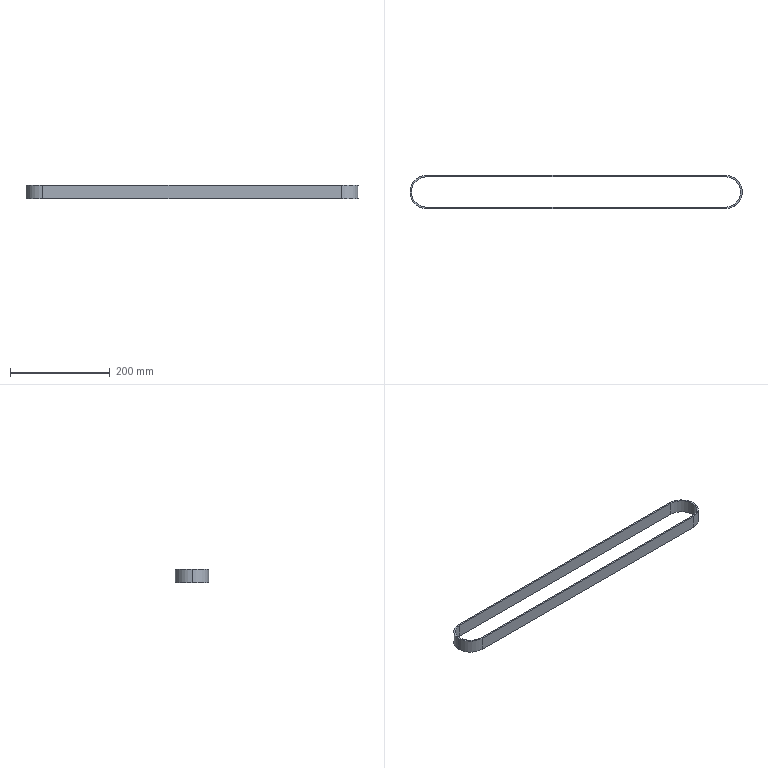Part | SolidWorks | features Extrusion 1 | 1 solid | 12 faces | box 667 x 67 x 27 mm | volume 113486 mm3 | cylinder 6 | plane 6 | commonest cylinder face diameters 61 x3 67 x3
STEP:
#1=CARTESIAN_POINT('',(0.,30.5,13.5));
#2=VERTEX_POINT('',#1);
#3=CARTESIAN_POINT('',(-30.5,0.,13.5));
#4=VERTEX_POINT('',#3);
#5=CARTESIAN_POINT('',(0.,0.,13.5));
#6=DIRECTION('',(0.,0.,1.));
#7=DIRECTION('',(1.,0.,0.));
#8=AXIS2_PLACEMENT_3D('',#5,#6,#7);
#9=CIRCLE('',#8,30.5);
#10=EDGE_CURVE('',#2,#4,#9,.T.);
#11=ORIENTED_EDGE('',*,*,#10,.T.);
#12=CARTESIAN_POINT('',(-30.5,0.,-13.5));
#13=VERTEX_POINT('',#12);
#14=CARTESIAN_POINT('',(-30.5,0.,13.5));
#15=DIRECTION('',(0.,0.,-1.));
#16=VECTOR('',#15,1000.);
#17=LINE('',#14,#16);
#18=EDGE_CURVE('',#4,#13,#17,.T.);
#19=ORIENTED_EDGE('',*,*,#18,.T.);
#20=CARTESIAN_POINT('',(0.,30.5,-13.5));
#21=VERTEX_POINT('',#20);
#22=CARTESIAN_POINT('',(0.,0.,-13.5));
#23=DIRECTION('',(0.,0.,1.));
#24=DIRECTION('',(1.,0.,0.));
#25=AXIS2_PLACEMENT_3D('',#22,#23,#24);
#26=CIRCLE('',#25,30.5);
#27=EDGE_CURVE('',#21,#13,#26,.T.);
#28=ORIENTED_EDGE('',*,*,#27,.F.);
#29=CARTESIAN_POINT('',(0.,30.5,13.5));
#30=DIRECTION('',(0.,0.,-1.));
#31=VECTOR('',#30,1000.);
#32=LINE('',#29,#31);
#33=EDGE_CURVE('',#2,#21,#32,.T.);
#34=ORIENTED_EDGE('',*,*,#33,.F.);
#35=EDGE_LOOP('',(#11,#19,#28,#34));
#36=FACE_OUTER_BOUND('',#35,.T.);
#37=CARTESIAN_POINT('',(0.,0.,13.5));
#38=DIRECTION('',(0.,0.,-1.));
#39=DIRECTION('',(-1.,0.,0.));
#40=AXIS2_PLACEMENT_3D('',#37,#38,#39);
#41=CYLINDRICAL_SURFACE('',#40,30.5);
#42=ADVANCED_FACE('',(#36),#41,.F.);
#43=CARTESIAN_POINT('',(-33.5,0.,13.5));
#44=VERTEX_POINT('',#43);
#45=CARTESIAN_POINT('',(0.,-33.5,13.5));
#46=VERTEX_POINT('',#45);
#47=CARTESIAN_POINT('',(0.,0.,13.5));
#48=DIRECTION('',(0.,0.,1.));
#49=DIRECTION('',(1.,0.,0.));
#50=AXIS2_PLACEMENT_3D('',#47,#48,#49);
#51=CIRCLE('',#50,33.5);
#52=EDGE_CURVE('',#44,#46,#51,.T.);
#53=ORIENTED_EDGE('',*,*,#52,.F.);
#54=CARTESIAN_POINT('',(-33.5,0.,-13.5));
#55=VERTEX_POINT('',#54);
#56=CARTESIAN_POINT('',(-33.5,0.,13.5));
#57=DIRECTION('',(0.,0.,-1.));
#58=VECTOR('',#57,1000.);
#59=LINE('',#56,#58);
#60=EDGE_CURVE('',#44,#55,#59,.T.);
#61=ORIENTED_EDGE('',*,*,#60,.T.);
#62=CARTESIAN_POINT('',(0.,-33.5,-13.5));
#63=VERTEX_POINT('',#62);
#64=CARTESIAN_POINT('',(0.,0.,-13.5));
#65=DIRECTION('',(0.,0.,1.));
#66=DIRECTION('',(1.,0.,0.));
#67=AXIS2_PLACEMENT_3D('',#64,#65,#66);
#68=CIRCLE('',#67,33.5);
#69=EDGE_CURVE('',#55,#63,#68,.T.);
#70=ORIENTED_EDGE('',*,*,#69,.T.);
#71=CARTESIAN_POINT('',(0.,-33.5,13.5));
#72=DIRECTION('',(0.,0.,-1.));
#73=VECTOR('',#72,1000.);
#74=LINE('',#71,#73);
#75=EDGE_CURVE('',#46,#63,#74,.T.);
#76=ORIENTED_EDGE('',*,*,#75,.F.);
#77=EDGE_LOOP('',(#53,#61,#70,#76));
#78=FACE_OUTER_BOUND('',#77,.T.);
#79=CARTESIAN_POINT('',(0.,0.,13.5));
#80=DIRECTION('',(0.,0.,-1.));
#81=DIRECTION('',(-1.,0.,0.));
#82=AXIS2_PLACEMENT_3D('',#79,#80,#81);
#83=CYLINDRICAL_SURFACE('',#82,33.5);
#84=ADVANCED_FACE('',(#78),#83,.T.);
#85=CARTESIAN_POINT('',(0.,33.5,13.5));
#86=VERTEX_POINT('',#85);
#87=CARTESIAN_POINT('',(0.,0.,13.5));
#88=DIRECTION('',(0.,0.,1.));
#89=DIRECTION('',(1.,0.,0.));
#90=AXIS2_PLACEMENT_3D('',#87,#88,#89);
#91=CIRCLE('',#90,33.5);
#92=EDGE_CURVE('',#86,#44,#91,.T.);
#93=ORIENTED_EDGE('',*,*,#92,.T.);
#94=ORIENTED_EDGE('',*,*,#52,.T.);
#95=CARTESIAN_POINT('',(600.,-33.5,13.5));
#96=VERTEX_POINT('',#95);
#97=CARTESIAN_POINT('',(0.,-33.5,13.5));
#98=DIRECTION('',(1.,0.,0.));
#99=VECTOR('',#98,1000.);
#100=LINE('',#97,#99);
#101=EDGE_CURVE('',#46,#96,#100,.T.);
#102=ORIENTED_EDGE('',*,*,#101,.T.);
#103=CARTESIAN_POINT('',(600.,33.5,13.5));
#104=VERTEX_POINT('',#103);
#105=CARTESIAN_POINT('',(600.,0.,13.5));
#106=DIRECTION('',(0.,0.,1.));
#107=DIRECTION('',(1.,0.,0.));
#108=AXIS2_PLACEMENT_3D('',#105,#106,#107);
#109=CIRCLE('',#108,33.5);
#110=EDGE_CURVE('',#96,#104,#109,.T.);
#111=ORIENTED_EDGE('',*,*,#110,.T.);
#112=CARTESIAN_POINT('',(0.,33.5,13.5));
#113=DIRECTION('',(-1.,0.,0.));
#114=VECTOR('',#113,1000.);
#115=LINE('',#112,#114);
#116=EDGE_CURVE('',#104,#86,#115,.T.);
#117=ORIENTED_EDGE('',*,*,#116,.T.);
#118=EDGE_LOOP('',(#93,#94,#102,#111,#117));
#119=FACE_OUTER_BOUND('',#118,.T.);
#120=CARTESIAN_POINT('',(0.,-30.5,13.5));
#121=VERTEX_POINT('',#120);
#122=CARTESIAN_POINT('',(600.,-30.5,13.5));
#123=VERTEX_POINT('',#122);
#124=CARTESIAN_POINT('',(0.,-30.5,13.5));
#125=DIRECTION('',(1.,0.,0.));
#126=VECTOR('',#125,1000.);
#127=LINE('',#124,#126);
#128=EDGE_CURVE('',#121,#123,#127,.T.);
#129=ORIENTED_EDGE('',*,*,#128,.F.);
#130=CARTESIAN_POINT('',(0.,0.,13.5));
#131=DIRECTION('',(0.,0.,1.));
#132=DIRECTION('',(1.,0.,0.));
#133=AXIS2_PLACEMENT_3D('',#130,#131,#132);
#134=CIRCLE('',#133,30.5);
#135=EDGE_CURVE('',#4,#121,#134,.T.);
#136=ORIENTED_EDGE('',*,*,#135,.F.);
#137=ORIENTED_EDGE('',*,*,#10,.F.);
#138=CARTESIAN_POINT('',(600.,30.5,13.5));
#139=VERTEX_POINT('',#138);
#140=CARTESIAN_POINT('',(0.,30.5,13.5));
#141=DIRECTION('',(-1.,0.,0.));
#142=VECTOR('',#141,1000.);
#143=LINE('',#140,#142);
#144=EDGE_CURVE('',#139,#2,#143,.T.);
#145=ORIENTED_EDGE('',*,*,#144,.F.);
#146=CARTESIAN_POINT('',(600.,0.,13.5));
#147=DIRECTION('',(0.,0.,1.));
#148=DIRECTION('',(1.,0.,0.));
#149=AXIS2_PLACEMENT_3D('',#146,#147,#148);
#150=CIRCLE('',#149,30.5);
#151=EDGE_CURVE('',#123,#139,#150,.T.);
#152=ORIENTED_EDGE('',*,*,#151,.F.);
#153=EDGE_LOOP('',(#129,#136,#137,#145,#152));
#154=FACE_BOUND('',#153,.T.);
#155=CARTESIAN_POINT('',(0.,0.,13.5));
#156=DIRECTION('',(0.,0.,1.));
#157=DIRECTION('',(1.,0.,0.));
#158=AXIS2_PLACEMENT_3D('',#155,#156,#157);
#159=PLANE('',#158);
#160=ADVANCED_FACE('',(#119,#154),#159,.T.);
#161=CARTESIAN_POINT('',(0.,33.5,-13.5));
#162=VERTEX_POINT('',#161);
#163=CARTESIAN_POINT('',(0.,0.,-13.5));
#164=DIRECTION('',(0.,0.,1.));
#165=DIRECTION('',(1.,0.,0.));
#166=AXIS2_PLACEMENT_3D('',#163,#164,#165);
#167=CIRCLE('',#166,33.5);
#168=EDGE_CURVE('',#162,#55,#167,.T.);
#169=ORIENTED_EDGE('',*,*,#168,.F.);
#170=CARTESIAN_POINT('',(600.,33.5,-13.5));
#171=VERTEX_POINT('',#170);
#172=CARTESIAN_POINT('',(0.,33.5,-13.5));
#173=DIRECTION('',(-1.,0.,0.));
#174=VECTOR('',#173,1000.);
#175=LINE('',#172,#174);
#176=EDGE_CURVE('',#171,#162,#175,.T.);
#177=ORIENTED_EDGE('',*,*,#176,.F.);
#178=CARTESIAN_POINT('',(600.,-33.5,-13.5));
#179=VERTEX_POINT('',#178);
#180=CARTESIAN_POINT('',(600.,0.,-13.5));
#181=DIRECTION('',(0.,0.,1.));
#182=DIRECTION('',(1.,0.,0.));
#183=AXIS2_PLACEMENT_3D('',#180,#181,#182);
#184=CIRCLE('',#183,33.5);
#185=EDGE_CURVE('',#179,#171,#184,.T.);
#186=ORIENTED_EDGE('',*,*,#185,.F.);
#187=CARTESIAN_POINT('',(0.,-33.5,-13.5));
#188=DIRECTION('',(1.,0.,0.));
#189=VECTOR('',#188,1000.);
#190=LINE('',#187,#189);
#191=EDGE_CURVE('',#63,#179,#190,.T.);
#192=ORIENTED_EDGE('',*,*,#191,.F.);
#193=ORIENTED_EDGE('',*,*,#69,.F.);
#194=EDGE_LOOP('',(#169,#177,#186,#192,#193));
#195=FACE_OUTER_BOUND('',#194,.T.);
#196=ORIENTED_EDGE('',*,*,#27,.T.);
#197=CARTESIAN_POINT('',(0.,-30.5,-13.5));
#198=VERTEX_POINT('',#197);
#199=CARTESIAN_POINT('',(0.,0.,-13.5));
#200=DIRECTION('',(0.,0.,1.));
#201=DIRECTION('',(1.,0.,0.));
#202=AXIS2_PLACEMENT_3D('',#199,#200,#201);
#203=CIRCLE('',#202,30.5);
#204=EDGE_CURVE('',#13,#198,#203,.T.);
#205=ORIENTED_EDGE('',*,*,#204,.T.);
#206=CARTESIAN_POINT('',(600.,-30.5,-13.5));
#207=VERTEX_POINT('',#206);
#208=CARTESIAN_POINT('',(0.,-30.5,-13.5));
#209=DIRECTION('',(1.,0.,0.));
#210=VECTOR('',#209,1000.);
#211=LINE('',#208,#210);
#212=EDGE_CURVE('',#198,#207,#211,.T.);
#213=ORIENTED_EDGE('',*,*,#212,.T.);
#214=CARTESIAN_POINT('',(600.,30.5,-13.5));
#215=VERTEX_POINT('',#214);
#216=CARTESIAN_POINT('',(600.,0.,-13.5));
#217=DIRECTION('',(0.,0.,1.));
#218=DIRECTION('',(1.,0.,0.));
#219=AXIS2_PLACEMENT_3D('',#216,#217,#218);
#220=CIRCLE('',#219,30.5);
#221=EDGE_CURVE('',#207,#215,#220,.T.);
#222=ORIENTED_EDGE('',*,*,#221,.T.);
#223=CARTESIAN_POINT('',(0.,30.5,-13.5));
#224=DIRECTION('',(-1.,0.,0.));
#225=VECTOR('',#224,1000.);
#226=LINE('',#223,#225);
#227=EDGE_CURVE('',#215,#21,#226,.T.);
#228=ORIENTED_EDGE('',*,*,#227,.T.);
#229=EDGE_LOOP('',(#196,#205,#213,#222,#228));
#230=FACE_BOUND('',#229,.T.);
#231=CARTESIAN_POINT('',(0.,0.,-13.5));
#232=DIRECTION('',(0.,0.,1.));
#233=DIRECTION('',(1.,0.,0.));
#234=AXIS2_PLACEMENT_3D('',#231,#232,#233);
#235=PLANE('',#234);
#236=ADVANCED_FACE('',(#195,#230),#235,.F.);
#237=ORIENTED_EDGE('',*,*,#60,.F.);
#238=ORIENTED_EDGE('',*,*,#92,.F.);
#239=CARTESIAN_POINT('',(0.,33.5,13.5));
#240=DIRECTION('',(0.,0.,-1.));
#241=VECTOR('',#240,1000.);
#242=LINE('',#239,#241);
#243=EDGE_CURVE('',#86,#162,#242,.T.);
#244=ORIENTED_EDGE('',*,*,#243,.T.);
#245=ORIENTED_EDGE('',*,*,#168,.T.);
#246=EDGE_LOOP('',(#237,#238,#244,#245));
#247=FACE_OUTER_BOUND('',#246,.T.);
#248=CARTESIAN_POINT('',(0.,0.,13.5));
#249=DIRECTION('',(0.,0.,-1.));
#250=DIRECTION('',(-1.,0.,0.));
#251=AXIS2_PLACEMENT_3D('',#248,#249,#250);
#252=CYLINDRICAL_SURFACE('',#251,33.5);
#253=ADVANCED_FACE('',(#247),#252,.T.);
#254=ORIENTED_EDGE('',*,*,#191,.T.);
#255=CARTESIAN_POINT('',(600.,-33.5,13.5));
#256=DIRECTION('',(0.,0.,-1.));
#257=VECTOR('',#256,1000.);
#258=LINE('',#255,#257);
#259=EDGE_CURVE('',#96,#179,#258,.T.);
#260=ORIENTED_EDGE('',*,*,#259,.F.);
#261=ORIENTED_EDGE('',*,*,#101,.F.);
#262=ORIENTED_EDGE('',*,*,#75,.T.);
#263=EDGE_LOOP('',(#254,#260,#261,#262));
#264=FACE_OUTER_BOUND('',#263,.T.);
#265=CARTESIAN_POINT('',(0.,-33.5,13.5));
#266=DIRECTION('',(0.,1.,0.));
#267=DIRECTION('',(0.,0.,1.));
#268=AXIS2_PLACEMENT_3D('',#265,#266,#267);
#269=PLANE('',#268);
#270=ADVANCED_FACE('',(#264),#269,.F.);
#271=ORIENTED_EDGE('',*,*,#185,.T.);
#272=CARTESIAN_POINT('',(600.,33.5,13.5));
#273=DIRECTION('',(0.,0.,-1.));
#274=VECTOR('',#273,1000.);
#275=LINE('',#272,#274);
#276=EDGE_CURVE('',#104,#171,#275,.T.);
#277=ORIENTED_EDGE('',*,*,#276,.F.);
#278=ORIENTED_EDGE('',*,*,#110,.F.);
#279=ORIENTED_EDGE('',*,*,#259,.T.);
#280=EDGE_LOOP('',(#271,#277,#278,#279));
#281=FACE_OUTER_BOUND('',#280,.T.);
#282=CARTESIAN_POINT('',(600.,0.,13.5));
#283=DIRECTION('',(0.,0.,-1.));
#284=DIRECTION('',(-1.,0.,0.));
#285=AXIS2_PLACEMENT_3D('',#282,#283,#284);
#286=CYLINDRICAL_SURFACE('',#285,33.5);
#287=ADVANCED_FACE('',(#281),#286,.T.);
#288=ORIENTED_EDGE('',*,*,#176,.T.);
#289=ORIENTED_EDGE('',*,*,#243,.F.);
#290=ORIENTED_EDGE('',*,*,#116,.F.);
#291=ORIENTED_EDGE('',*,*,#276,.T.);
#292=EDGE_LOOP('',(#288,#289,#290,#291));
#293=FACE_OUTER_BOUND('',#292,.T.);
#294=CARTESIAN_POINT('',(0.,33.5,13.5));
#295=DIRECTION('',(0.,-1.,0.));
#296=DIRECTION('',(0.,0.,-1.));
#297=AXIS2_PLACEMENT_3D('',#294,#295,#296);
#298=PLANE('',#297);
#299=ADVANCED_FACE('',(#293),#298,.F.);
#300=ORIENTED_EDGE('',*,*,#18,.F.);
#301=ORIENTED_EDGE('',*,*,#135,.T.);
#302=CARTESIAN_POINT('',(0.,-30.5,13.5));
#303=DIRECTION('',(0.,0.,-1.));
#304=VECTOR('',#303,1000.);
#305=LINE('',#302,#304);
#306=EDGE_CURVE('',#121,#198,#305,.T.);
#307=ORIENTED_EDGE('',*,*,#306,.T.);
#308=ORIENTED_EDGE('',*,*,#204,.F.);
#309=EDGE_LOOP('',(#300,#301,#307,#308));
#310=FACE_OUTER_BOUND('',#309,.T.);
#311=CARTESIAN_POINT('',(0.,0.,13.5));
#312=DIRECTION('',(0.,0.,-1.));
#313=DIRECTION('',(-1.,0.,0.));
#314=AXIS2_PLACEMENT_3D('',#311,#312,#313);
#315=CYLINDRICAL_SURFACE('',#314,30.5);
#316=ADVANCED_FACE('',(#310),#315,.F.);
#317=ORIENTED_EDGE('',*,*,#212,.F.);
#318=ORIENTED_EDGE('',*,*,#306,.F.);
#319=ORIENTED_EDGE('',*,*,#128,.T.);
#320=CARTESIAN_POINT('',(600.,-30.5,13.5));
#321=DIRECTION('',(0.,0.,-1.));
#322=VECTOR('',#321,1000.);
#323=LINE('',#320,#322);
#324=EDGE_CURVE('',#123,#207,#323,.T.);
#325=ORIENTED_EDGE('',*,*,#324,.T.);
#326=EDGE_LOOP('',(#317,#318,#319,#325));
#327=FACE_OUTER_BOUND('',#326,.T.);
#328=CARTESIAN_POINT('',(0.,-30.5,13.5));
#329=DIRECTION('',(0.,1.,0.));
#330=DIRECTION('',(0.,0.,1.));
#331=AXIS2_PLACEMENT_3D('',#328,#329,#330);
#332=PLANE('',#331);
#333=ADVANCED_FACE('',(#327),#332,.T.);
#334=ORIENTED_EDGE('',*,*,#221,.F.);
#335=ORIENTED_EDGE('',*,*,#324,.F.);
#336=ORIENTED_EDGE('',*,*,#151,.T.);
#337=CARTESIAN_POINT('',(600.,30.5,13.5));
#338=DIRECTION('',(0.,0.,-1.));
#339=VECTOR('',#338,1000.);
#340=LINE('',#337,#339);
#341=EDGE_CURVE('',#139,#215,#340,.T.);
#342=ORIENTED_EDGE('',*,*,#341,.T.);
#343=EDGE_LOOP('',(#334,#335,#336,#342));
#344=FACE_OUTER_BOUND('',#343,.T.);
#345=CARTESIAN_POINT('',(600.,0.,13.5));
#346=DIRECTION('',(0.,0.,-1.));
#347=DIRECTION('',(-1.,0.,0.));
#348=AXIS2_PLACEMENT_3D('',#345,#346,#347);
#349=CYLINDRICAL_SURFACE('',#348,30.5);
#350=ADVANCED_FACE('',(#344),#349,.F.);
#351=ORIENTED_EDGE('',*,*,#227,.F.);
#352=ORIENTED_EDGE('',*,*,#341,.F.);
#353=ORIENTED_EDGE('',*,*,#144,.T.);
#354=ORIENTED_EDGE('',*,*,#33,.T.);
#355=EDGE_LOOP('',(#351,#352,#353,#354));
#356=FACE_OUTER_BOUND('',#355,.T.);
#357=CARTESIAN_POINT('',(0.,30.5,13.5));
#358=DIRECTION('',(0.,-1.,0.));
#359=DIRECTION('',(0.,0.,-1.));
#360=AXIS2_PLACEMENT_3D('',#357,#358,#359);
#361=PLANE('',#360);
#362=ADVANCED_FACE('',(#356),#361,.T.);
#363=CLOSED_SHELL('',(#42,#84,#160,#236,#253,#270,#287,#299,#316,#333,#350,#362));
#364=MANIFOLD_SOLID_BREP('',#363);
#365=CARTESIAN_POINT('',(0.,0.,0.));
#366=DIRECTION('',(0.,0.,1.));
#367=DIRECTION('',(1.,0.,0.));
#368=AXIS2_PLACEMENT_3D('',#365,#366,#367);
#369=(LENGTH_UNIT()NAMED_UNIT(*)SI_UNIT(.MILLI.,.METRE.));
#370=UNCERTAINTY_MEASURE_WITH_UNIT(LENGTH_MEASURE(0.00001),#369,'','');
#371=(NAMED_UNIT(*)PLANE_ANGLE_UNIT()SI_UNIT($,.RADIAN.));
#372=(NAMED_UNIT(*)SI_UNIT($,.STERADIAN.)SOLID_ANGLE_UNIT());
#373=(GEOMETRIC_REPRESENTATION_CONTEXT(3)GLOBAL_UNCERTAINTY_ASSIGNED_CONTEXT((#370))GLOBAL_UNIT_ASSIGNED_CONTEXT((#369,#371,#372))REPRESENTATION_CONTEXT('',''));
#374=ADVANCED_BREP_SHAPE_REPRESENTATION('',(#364,#368),#373);